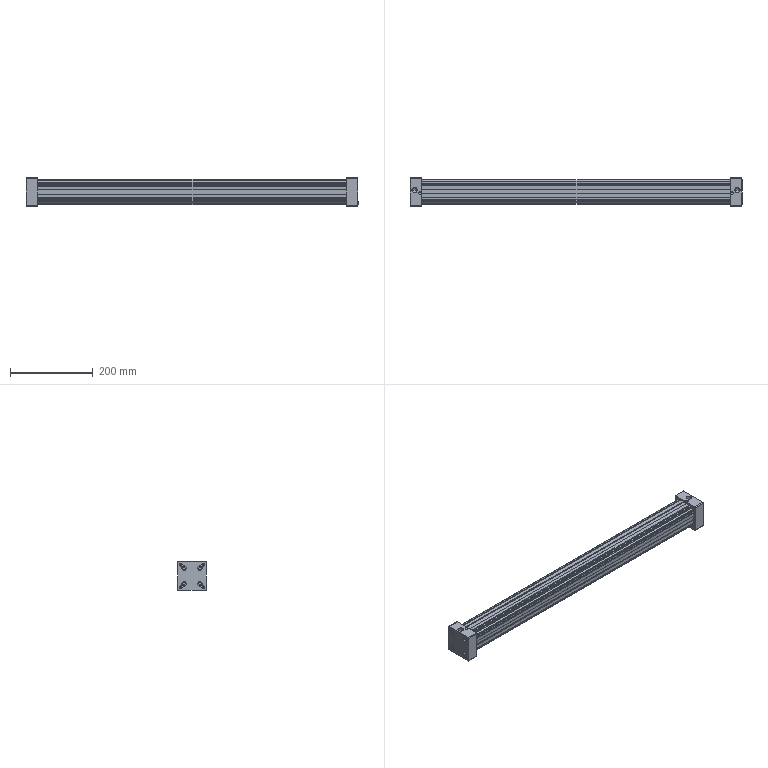Part | STEP file | HI_PRU40500b | 1 solid | 290 faces | box 800 x 69 x 69 mm | volume 2639652 mm3 | plane 134 | cylinder 116 | cone 40 | commonest cylinder face diameters 1 x24 2 x22 4.917 x16 10 x16 11 x16 4 x8